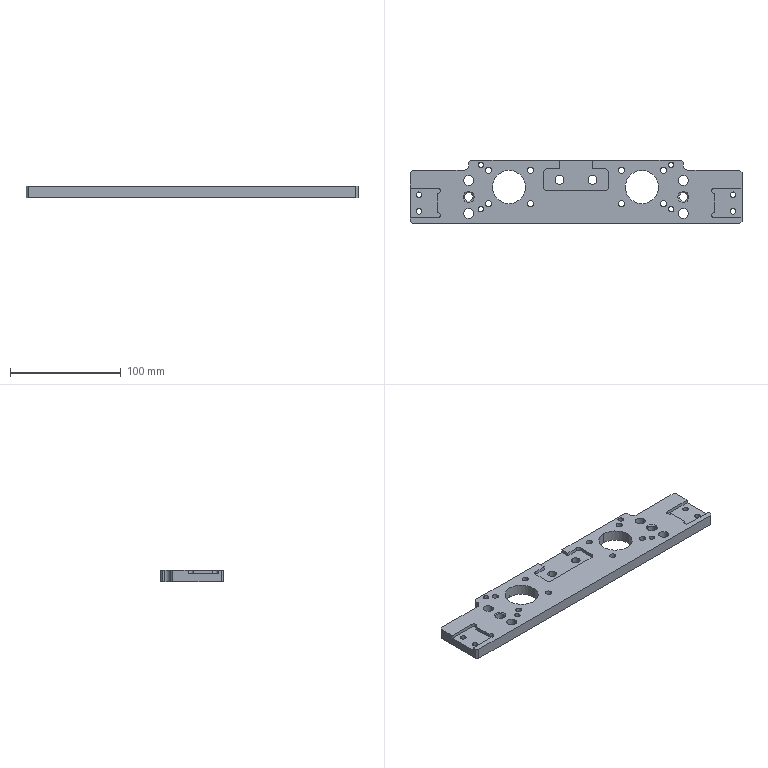Part | STEP file | J454-EBZ05-26-00-Part-1-1 | 1 solid | 134 faces | box 300 x 57 x 10 mm | volume 129262 mm3 | cylinder 86 | plane 44 | cone 4 | commonest cylinder face diameters 5 x20 5.5 x16 9.5 x16 4.5 x8 8 x8 9 x8